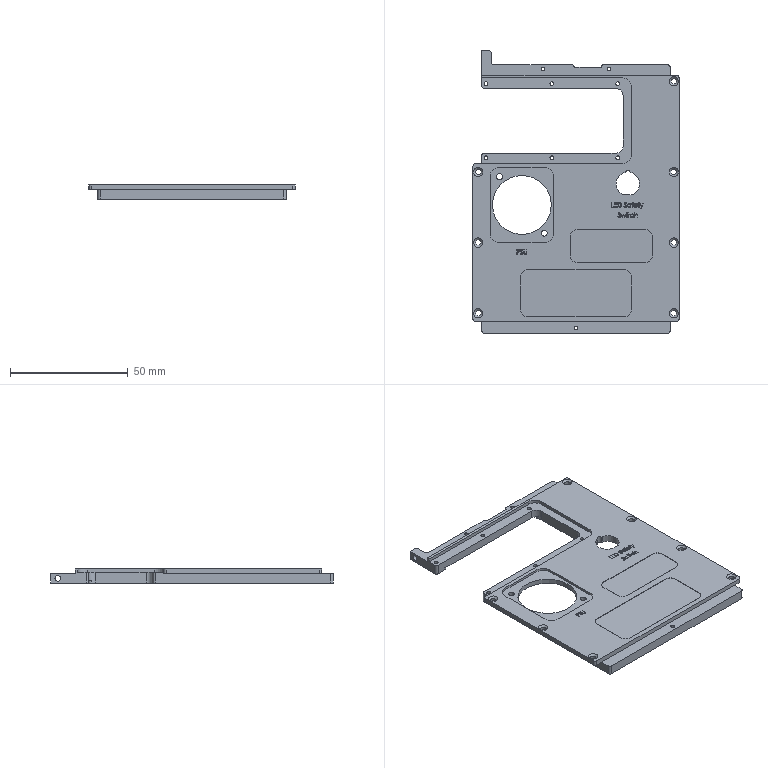Part | 1 solid | 481 faces | box 87.5 x 120 x 6.001 mm | volume 22892 mm3 | plane 247 | cylinder 121 | spline 106 | cone 7 | commonest cylinder face diameters 2 x77 6 x10 1.6 x9 2.4 x8 1 x6 8 x6